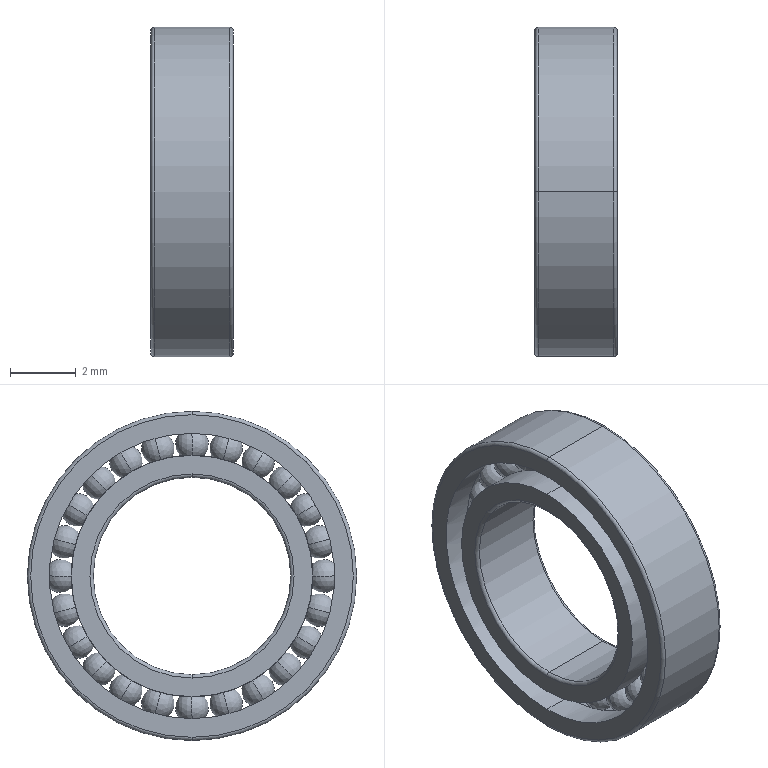Part | SolidWorks | features Stock 1 | 1 solid | 144 faces | box 2.5 x 10 x 10 mm | volume 92.163 mm3 | torus 80 | sphere 48 | cylinder 12 | plane 4 | commonest cylinder face diameters 7.333 x4 8.667 x4 6 x2 10 x2